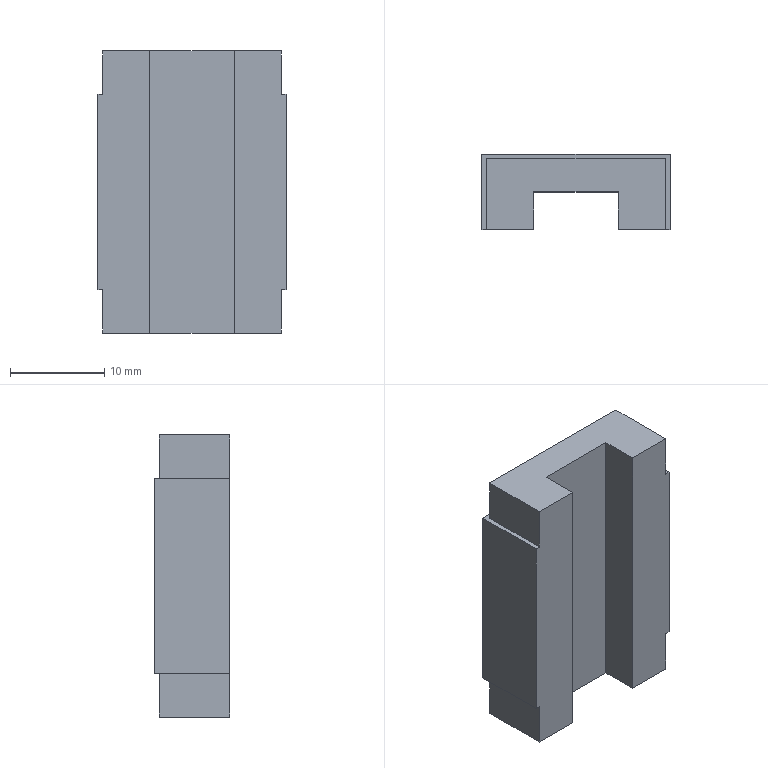Part | STEP file | SOLID | 1 solid | 34 faces | box 20 x 8 x 30 mm | volume 3476 mm3 | plane 18 | cone 8 | cylinder 8 | commonest cylinder face diameters 2.5 x8